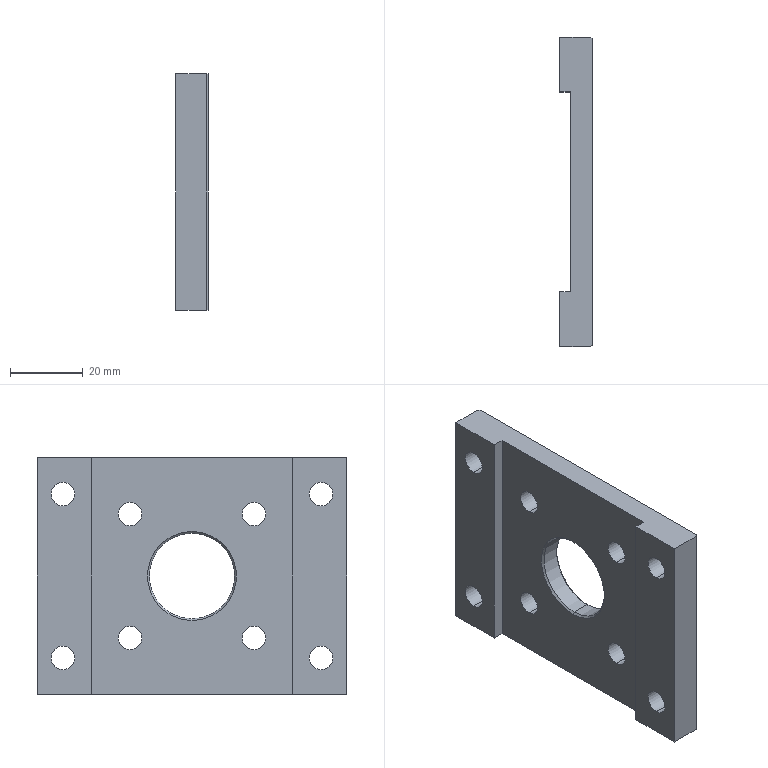Part | STEP file | 1 solid | 34 faces | box 9 x 85 x 65 mm | volume 34372 mm3 | cylinder 18 | plane 12 | cone 4 | commonest cylinder face diameters 6.5 x16 23.5 x2